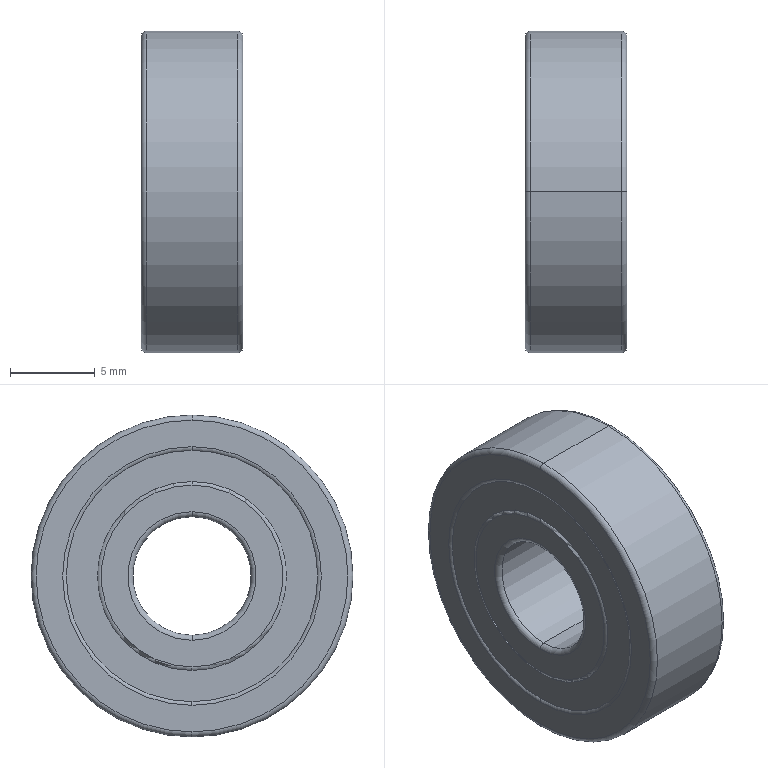Part | SolidWorks | features Revolution 5, CirPattern 2, RefAxis 1, RevCut 1 | 12 solids | 148 faces | box 6 x 19 x 19 mm | volume 1166 mm3 | cylinder 50 | sphere 44 | plane 28 | torus 26 | commonest cylinder face diameters 11.85 x19 13.15 x19 11.333 x4 14.667 x4 7 x2 19 x2